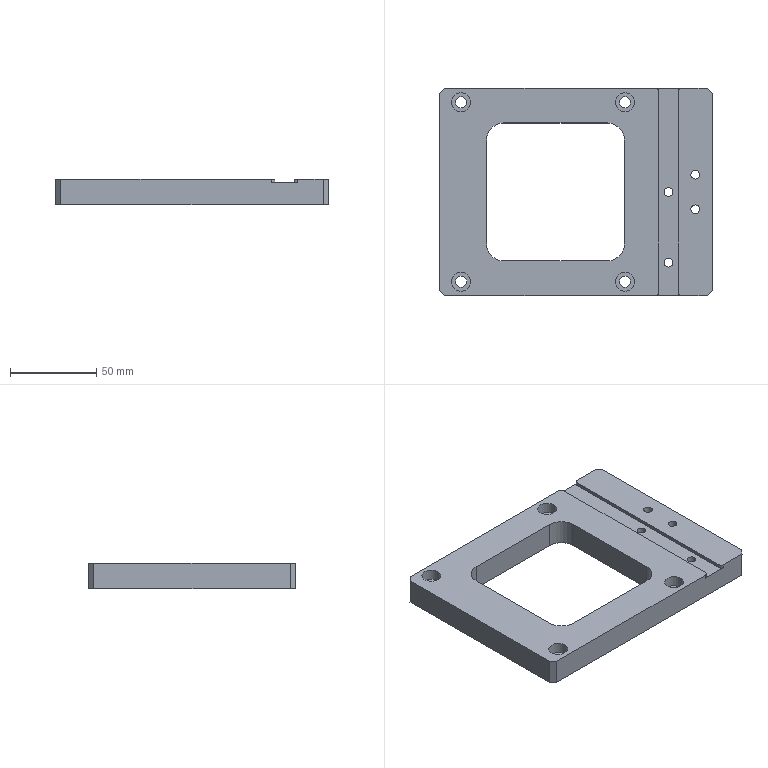CAM job | NX | 3-axis milling, drilling | part box 158.2 x 120 x 15 mm | stock box 163.2 x 125 x 20 mm
Tools:
number,name,description,diameter,corner_radius,flute_length,length,flutes
6,D6,平底铣刀-粗,6.0,0.0,25.0,75.0,2
9,D10,平底铣刀-粗,10.0,0.0,35.0,75.0,2
7,D6-J,平底铣刀-精,6.0,0.0,25.0,75.0,2
10,D10-J,平底铣刀-精,10.0,0.0,35.0,75.0,2
1,D80R0.8飞刀,圆鼻刀-粗,80.0,0.8,50.0,75.0,2
1,D80R0.8飞刀-J,圆鼻刀-精,80.0,0.8,50.0,75.0,2
2,D6倒角刀,倒角刀,6.0,0.0,3.0,25.0,2
18,M6X1.0,丝锥,5.0,0.0,35.0,50.0,2
15,ZT5,钻头,5.0,0.0,35.0,50.0,2
17,ZT6.5,钻头,6.5,0.0,35.0,50.0,2
Operations:
program,operation,operation_type,tool,method,geometry_group,spindle_rpm,surface_speed,feed_per_tooth,feed_cut,feed_plunge,cut_length_mm,path_length_mm,cut_time_min,machine_time_min
B,底壁铣飞面开粗_COPY,VolumeBased25DMillingOperation,D80R0.8飞刀,分层开粗-切深K-步距G,W-B,2800.0,703.696,0.5357,3000.0,100.0,3376.525,3734.084,1.125,1.161
B,底壁铣飞面精光_COPY,VolumeBased25DMillingOperation,D80R0.8飞刀-J,侧刃精光-切深K-步距G,W-B,4000.0,1005.28,0.125,1000.0,100.0,794.184,830.184,0.7942,0.7978
B,铣倒角_4,PlanarMilling,D6倒角刀,METHOD,W-B,6000.0,113.097,0.05,600.0,100.0,75.821,311.262,0.1264,0.1499
B,铣倒角_5,PlanarMilling,D6倒角刀,METHOD,W-B,6000.0,113.097,0.05,600.0,100.0,80.763,544.12,0.1346,0.1809
B,C0.3封闭铣廓倒角6X45L_COPY,PlanarMilling,D6倒角刀,爬面_倒角-切深0-步距G,W-B,7000.0,131.0,0.1071,1500.0,100.0,878.566,1033.725,0.5857,0.6012
A,顶面,FaceMilling,D80R0.8飞刀,侧刃精光-切深K-步距G,W-A,4000.0,1005.31,0.125,1000.0,100.0,828.6,864.6,0.8286,0.8322
A,外形粗_2,VolumeBased25DMillingOperation,D10,METHOD,W-A,8000.0,251.327,0.3125,5000.0,80.0,12211.222,12264.922,2.442,2.448
A,框开粗_1,VolumeBased25DMillingOperation,D10,METHOD,W-A,6000.0,188.0,0.25,4000.0,80.0,8666.718,8720.067,2.167,2.172
A,底壁粗_1,VolumeBased25DMillingOperation,D6,METHOD,W-A,6000.0,113.0,0.2083,3500.0,100.0,1049.853,1111.772,0.3,0.3061
A,打点-深0.8,Operation,D6倒角刀,NONE,W-A,8000.0,150.796,0.0312,500.0,90.0,14.4,423.768,0.0288,0.0697
A,打点-深0.8_2,Operation,D6倒角刀,NONE,W-A,8000.0,150.796,0.0312,500.0,90.0,7.2,134.787,0.0144,0.0272
A,通孔-M6螺纹底孔,Operation,ZT5,NONE,W-A,2800.0,43.982,0.0625,350.0,90.0,90.009,300.404,0.2572,0.2782
A,沉头孔-钻孔0段,Operation,ZT6.5,NONE,W-A,1200.0,24.504,0.0625,150.0,90.0,79.811,496.638,0.5321,0.5738
A,铣孔开粗D6_1,CylinderMilling,D6,NONE,W-A,8000.0,150.796,0.075,1200.0,100.0,467.701,654.701,0.3898,0.4085
A,铣孔开粗D6_2,CylinderMilling,D6,NONE,W-A,8000.0,150.796,0.075,1200.0,100.0,467.701,654.701,0.3898,0.4085
A,仅选体,SurfaceContour,D6倒角刀,METHOD,W-A,8000.0,150.796,0.1875,3000.0,100.0,1139.584,1685.407,0.3799,0.4344
A,铣倒角_1,PlanarMilling,D6倒角刀,METHOD,W-A,8000.0,150.796,0.0312,500.0,100.0,36.963,140.532,0.0739,0.0843
A,铣倒角_2,PlanarMilling,D6倒角刀,NONE,W-A,8000.0,150.796,0.05,800.0,100.0,173.57,616.887,0.217,0.2613
A,铣倒角_3,PlanarMilling,D6倒角刀,METHOD,W-A,8000.0,150.796,0.0312,500.0,100.0,135.082,368.596,0.2702,0.2935
A,铣孔精光D6_1,CylinderMilling,D6-J,精光步距切深关,W-A,8000.0,150.796,0.0312,500.0,100.0,89.89,277.89,0.1798,0.1986
A,铣孔精光D6_2,CylinderMilling,D6-J,精光步距切深关,W-A,8000.0,150.796,0.0312,500.0,100.0,89.89,277.89,0.1798,0.1986
A,底侧精_3,VolumeBased25DMillingOperation,D6-J,METHOD,W-A,6000.0,113.0,0.2083,1200.0,100.0,282.899,391.399,0.2357,0.2466
A,框精_1,VolumeBased25DMillingOperation,D6-J,METHOD,W-A,6000.0,113.0,0.0833,1000.0,100.0,288.908,357.608,0.2889,0.2958
A,通孔-攻牙M6,Operation,M6X1.0,METHOD,W-A,500.0,7.854,0.001,1.0,90.0,78.0,272.171,78.0,78.019
A,外形半精_2,VolumeBased25DMillingOperation,D10-J,METHOD,W-A,8000.0,251.327,0.0625,1000.0,100.0,585.745,655.145,0.5857,0.5927